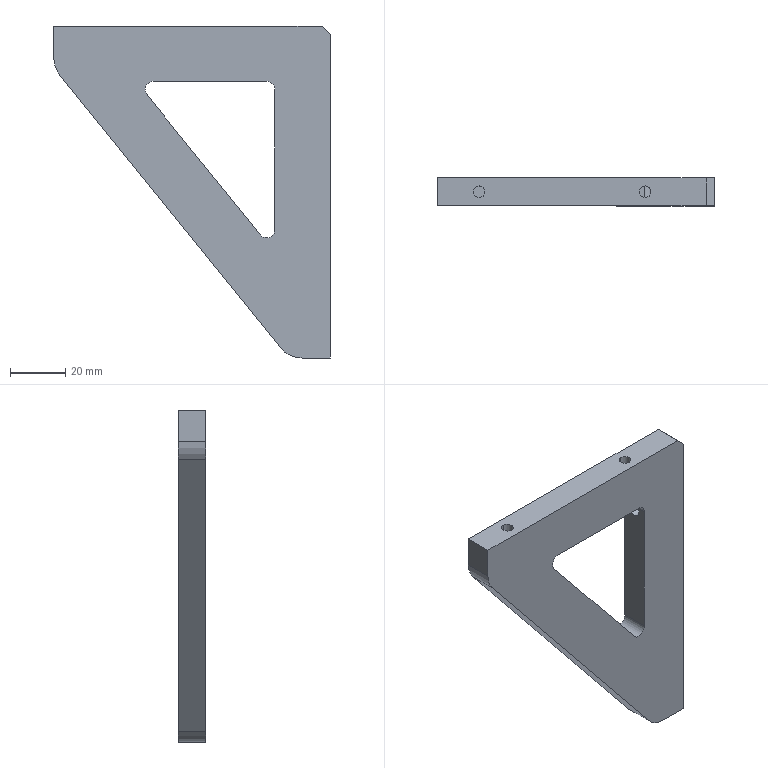Part | STEP file | PN_0006 | 1 solid | 26 faces | box 100 x 10 x 120 mm | volume 58710 mm3 | plane 13 | cylinder 13 | commonest cylinder face diameters 4.2 x8 6 x3 20 x2